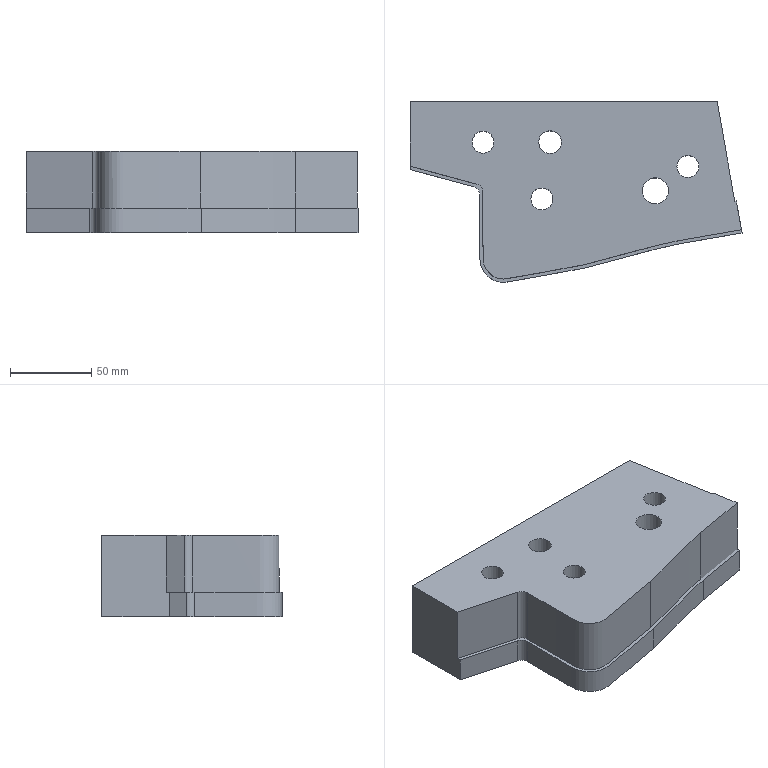Part | NX | features solid 2 | 1 solid | 32 faces | box 204.747 x 111.347 x 50 mm | volume 704636 mm3 | plane 16 | cylinder 10 | spline 6 | commonest cylinder face diameters 13.5 x3 19.5 x3 10 x2 14 x1 16 x1
STEP:
#1=CARTESIAN_POINT('',(-1121.897,435.,3.));
#2=VERTEX_POINT('',#1);
#3=CARTESIAN_POINT('',(-1121.897,435.,43.));
#4=VERTEX_POINT('',#3);
#5=CARTESIAN_POINT('',(-1121.897,435.,-60.));
#6=DIRECTION('',(0.,0.,-1.));
#7=VECTOR('',#6,1000.);
#8=LINE('',#5,#7);
#9=EDGE_CURVE('',#2,#4,#8,.F.);
#10=ORIENTED_EDGE('',*,*,#9,.F.);
#11=CARTESIAN_POINT('',(-1243.358,435.,3.));
#12=VERTEX_POINT('',#11);
#13=CARTESIAN_POINT('',(-1263.358,435.,3.));
#14=DIRECTION('',(-1.,0.,0.));
#15=VECTOR('',#14,1000.);
#16=LINE('',#13,#15);
#17=EDGE_CURVE('',#12,#2,#16,.F.);
#18=ORIENTED_EDGE('',*,*,#17,.F.);
#19=CARTESIAN_POINT('',(-1243.358,435.,-7.));
#20=VERTEX_POINT('',#19);
#21=CARTESIAN_POINT('',(-1243.358,435.,3.));
#22=DIRECTION('',(0.,0.,1.));
#23=VECTOR('',#22,1000.);
#24=LINE('',#21,#23);
#25=EDGE_CURVE('',#12,#20,#24,.F.);
#26=ORIENTED_EDGE('',*,*,#25,.T.);
#27=CARTESIAN_POINT('',(-1311.358,435.,-7.));
#28=VERTEX_POINT('',#27);
#29=CARTESIAN_POINT('',(-1263.358,435.,-7.));
#30=DIRECTION('',(-1.,0.,0.));
#31=VECTOR('',#30,1000.);
#32=LINE('',#29,#31);
#33=EDGE_CURVE('',#28,#20,#32,.F.);
#34=ORIENTED_EDGE('',*,*,#33,.F.);
#35=CARTESIAN_POINT('',(-1311.358,435.,43.));
#36=VERTEX_POINT('',#35);
#37=CARTESIAN_POINT('',(-1311.358,435.,-60.));
#38=DIRECTION('',(0.,0.,-1.));
#39=VECTOR('',#38,1000.);
#40=LINE('',#37,#39);
#41=EDGE_CURVE('',#36,#28,#40,.T.);
#42=ORIENTED_EDGE('',*,*,#41,.F.);
#43=CARTESIAN_POINT('',(-1263.358,435.,43.));
#44=DIRECTION('',(-1.,0.,0.));
#45=VECTOR('',#44,1000.);
#46=LINE('',#43,#45);
#47=EDGE_CURVE('',#36,#4,#46,.F.);
#48=ORIENTED_EDGE('',*,*,#47,.T.);
#49=EDGE_LOOP('',(#10,#18,#26,#34,#42,#48));
#50=FACE_BOUND('',#49,.T.);
#51=CARTESIAN_POINT('',(-1263.358,435.,-60.));
#52=DIRECTION('',(0.,1.,0.));
#53=DIRECTION('',(-1.,0.,0.));
#54=AXIS2_PLACEMENT_3D('',#51,#52,#53);
#55=PLANE('',#54);
#56=ADVANCED_FACE('',(#50),#55,.T.);
#57=CARTESIAN_POINT('',(-1266.355,379.299,8.));
#58=VERTEX_POINT('',#57);
#59=CARTESIAN_POINT('',(-1203.794,334.49,8.));
#60=VERTEX_POINT('',#59);
#61=CARTESIAN_POINT('',(-1266.355,379.299,8.));
#62=CARTESIAN_POINT('',(-1266.355,376.959,8.));
#63=CARTESIAN_POINT('',(-1266.356,372.279,8.));
#64=CARTESIAN_POINT('',(-1266.359,365.259,8.));
#65=CARTESIAN_POINT('',(-1266.363,358.239,8.));
#66=CARTESIAN_POINT('',(-1266.367,352.389,8.));
#67=CARTESIAN_POINT('',(-1266.372,347.71,8.));
#68=CARTESIAN_POINT('',(-1266.376,344.199,8.));
#69=CARTESIAN_POINT('',(-1266.38,340.694,8.));
#70=CARTESIAN_POINT('',(-1266.398,337.165,8.));
#71=CARTESIAN_POINT('',(-1265.599,333.731,8.));
#72=CARTESIAN_POINT('',(-1263.894,330.627,8.));
#73=CARTESIAN_POINT('',(-1261.439,328.077,8.));
#74=CARTESIAN_POINT('',(-1258.382,326.304,8.));
#75=CARTESIAN_POINT('',(-1254.93,325.476,8.));
#76=CARTESIAN_POINT('',(-1251.442,325.852,8.));
#77=CARTESIAN_POINT('',(-1248.056,326.515,8.));
#78=CARTESIAN_POINT('',(-1243.504,327.281,8.));
#79=CARTESIAN_POINT('',(-1237.826,328.278,8.));
#80=CARTESIAN_POINT('',(-1231.005,329.449,8.));
#81=CARTESIAN_POINT('',(-1224.186,330.621,8.));
#82=CARTESIAN_POINT('',(-1215.094,332.188,8.));
#83=CARTESIAN_POINT('',(-1208.297,333.483,8.));
#84=CARTESIAN_POINT('',(-1203.794,334.49,8.));
#85=B_SPLINE_CURVE_WITH_KNOTS('',3,(#61,#62,#63,#64,#65,#66,#67,#68,#69,#70,#71,#72,#73,#74,#75,#76,#77,#78,#79,#80,#81,#82,#83,#84),.UNSPECIFIED.,.F.,.F.,(4,1,1,1,1,1,1,1,1,1,1,1,1,1,1,1,1,1,1,1,1,4),(0.0507,0.05772,0.06474,0.07176,0.07878,0.08229,0.0858,0.08931,0.09282,0.09633,0.09984,0.1033,0.1069,0.1104,0.1139,0.1174,0.1209,0.1279,0.1349,0.142,0.149,0.163),.UNSPECIFIED.);
#86=EDGE_CURVE('',#58,#60,#85,.T.);
#87=ORIENTED_EDGE('',*,*,#86,.F.);
#88=CARTESIAN_POINT('',(-1270.061,384.129,8.));
#89=VERTEX_POINT('',#88);
#90=CARTESIAN_POINT('',(-1271.355,379.3,8.));
#91=DIRECTION('',(0.,0.,1.));
#92=DIRECTION('',(1.,0.,0.));
#93=AXIS2_PLACEMENT_3D('',#90,#91,#92);
#94=CIRCLE('',#93,5.);
#95=EDGE_CURVE('',#58,#89,#94,.T.);
#96=ORIENTED_EDGE('',*,*,#95,.T.);
#97=CARTESIAN_POINT('',(-1311.358,395.195,8.));
#98=VERTEX_POINT('',#97);
#99=CARTESIAN_POINT('',(-1243.118,376.91,8.));
#100=DIRECTION('',(0.9659,-0.2588,0.));
#101=VECTOR('',#100,1000.);
#102=LINE('',#99,#101);
#103=EDGE_CURVE('',#89,#98,#102,.F.);
#104=ORIENTED_EDGE('',*,*,#103,.T.);
#105=CARTESIAN_POINT('',(-1311.358,393.124,8.));
#106=VERTEX_POINT('',#105);
#107=CARTESIAN_POINT('',(-1311.358,338.697,8.));
#108=DIRECTION('',(0.,1.,0.));
#109=VECTOR('',#108,1000.);
#110=LINE('',#107,#109);
#111=EDGE_CURVE('',#98,#106,#110,.F.);
#112=ORIENTED_EDGE('',*,*,#111,.T.);
#113=CARTESIAN_POINT('',(-1272.064,382.595,8.));
#114=VERTEX_POINT('',#113);
#115=CARTESIAN_POINT('',(-1318.358,395.,8.));
#116=DIRECTION('',(0.9659,-0.2588,0.));
#117=VECTOR('',#116,1000.);
#118=LINE('',#115,#117);
#119=EDGE_CURVE('',#114,#106,#118,.F.);
#120=ORIENTED_EDGE('',*,*,#119,.F.);
#121=CARTESIAN_POINT('',(-1268.358,377.765,8.));
#122=VERTEX_POINT('',#121);
#123=CARTESIAN_POINT('',(-1273.358,377.766,8.));
#124=DIRECTION('',(0.,0.,1.));
#125=DIRECTION('',(1.,0.,0.));
#126=AXIS2_PLACEMENT_3D('',#123,#124,#125);
#127=CIRCLE('',#126,5.);
#128=EDGE_CURVE('',#114,#122,#127,.F.);
#129=ORIENTED_EDGE('',*,*,#128,.T.);
#130=CARTESIAN_POINT('',(-1203.358,332.538,8.));
#131=VERTEX_POINT('',#130);
#132=CARTESIAN_POINT('',(-1268.358,377.765,8.));
#133=CARTESIAN_POINT('',(-1268.358,375.398,8.));
#134=CARTESIAN_POINT('',(-1268.359,370.662,8.));
#135=CARTESIAN_POINT('',(-1268.362,363.558,8.));
#136=CARTESIAN_POINT('',(-1268.362,356.456,8.));
#137=CARTESIAN_POINT('',(-1268.38,349.349,8.));
#138=CARTESIAN_POINT('',(-1268.342,342.262,8.));
#139=CARTESIAN_POINT('',(-1268.525,335.095,8.));
#140=CARTESIAN_POINT('',(-1265.854,329.641,8.));
#141=CARTESIAN_POINT('',(-1262.445,326.353,8.));
#142=CARTESIAN_POINT('',(-1259.354,324.562,8.));
#143=CARTESIAN_POINT('',(-1255.924,323.61,8.));
#144=CARTESIAN_POINT('',(-1252.369,323.625,8.));
#145=CARTESIAN_POINT('',(-1248.874,324.351,8.));
#146=CARTESIAN_POINT('',(-1245.366,324.93,8.));
#147=CARTESIAN_POINT('',(-1241.862,325.548,8.));
#148=CARTESIAN_POINT('',(-1237.188,326.357,8.));
#149=CARTESIAN_POINT('',(-1229.008,327.775,8.));
#150=CARTESIAN_POINT('',(-1217.313,329.745,8.));
#151=CARTESIAN_POINT('',(-1207.99,331.502,8.));
#152=CARTESIAN_POINT('',(-1203.358,332.538,8.));
#153=B_SPLINE_CURVE_WITH_KNOTS('',3,(#132,#133,#134,#135,#136,#137,#138,#139,#140,#141,#142,#143,#144,#145,#146,#147,#148,#149,#150,#151,#152),.UNSPECIFIED.,.F.,.F.,(4,1,1,1,1,1,1,1,1,1,1,1,1,1,1,1,1,1,4),(0.05223,0.05934,0.06644,0.07354,0.08065,0.08775,0.09485,0.102,0.1055,0.1091,0.1126,0.1162,0.1197,0.1233,0.1268,0.1304,0.1375,0.1517,0.1659),.UNSPECIFIED.);
#154=EDGE_CURVE('',#122,#131,#153,.T.);
#155=ORIENTED_EDGE('',*,*,#154,.T.);
#156=CARTESIAN_POINT('',(-1145.033,347.385,8.));
#157=VERTEX_POINT('',#156);
#158=CARTESIAN_POINT('',(-1145.033,347.385,8.));
#159=CARTESIAN_POINT('',(-1154.893,345.514,8.));
#160=CARTESIAN_POINT('',(-1174.32,340.449,8.));
#161=CARTESIAN_POINT('',(-1193.559,334.73,8.));
#162=CARTESIAN_POINT('',(-1203.358,332.538,8.));
#163=B_SPLINE_CURVE_WITH_KNOTS('',3,(#158,#159,#160,#161,#162),.UNSPECIFIED.,.F.,.F.,(4,1,4),(0.,0.03009,0.06019),.UNSPECIFIED.);
#164=EDGE_CURVE('',#157,#131,#163,.T.);
#165=ORIENTED_EDGE('',*,*,#164,.F.);
#166=CARTESIAN_POINT('',(-1106.611,354.067,8.));
#167=VERTEX_POINT('',#166);
#168=CARTESIAN_POINT('',(-1145.033,347.385,8.));
#169=CARTESIAN_POINT('',(-1132.226,349.613,8.));
#170=CARTESIAN_POINT('',(-1119.418,351.84,8.));
#171=CARTESIAN_POINT('',(-1106.611,354.067,8.));
#172=B_SPLINE_CURVE_WITH_KNOTS('',3,(#168,#169,#170,#171),.UNSPECIFIED.,.F.,.F.,(4,4),(1.708,1.747),.UNSPECIFIED.);
#173=EDGE_CURVE('',#157,#167,#172,.T.);
#174=ORIENTED_EDGE('',*,*,#173,.T.);
#175=CARTESIAN_POINT('',(-1106.959,356.038,8.));
#176=VERTEX_POINT('',#175);
#177=CARTESIAN_POINT('',(-1108.407,364.255,8.));
#178=DIRECTION('',(0.1736,-0.9848,0.));
#179=VECTOR('',#178,1000.);
#180=LINE('',#177,#179);
#181=EDGE_CURVE('',#176,#167,#180,.T.);
#182=ORIENTED_EDGE('',*,*,#181,.F.);
#183=CARTESIAN_POINT('',(-1145.406,349.351,8.));
#184=VERTEX_POINT('',#183);
#185=CARTESIAN_POINT('',(-1145.406,349.351,8.));
#186=CARTESIAN_POINT('',(-1132.59,351.58,8.));
#187=CARTESIAN_POINT('',(-1119.774,353.809,8.));
#188=CARTESIAN_POINT('',(-1106.959,356.038,8.));
#189=B_SPLINE_CURVE_WITH_KNOTS('',3,(#185,#186,#187,#188),.UNSPECIFIED.,.F.,.F.,(4,4),(1.656,1.695),.UNSPECIFIED.);
#190=EDGE_CURVE('',#184,#176,#189,.T.);
#191=ORIENTED_EDGE('',*,*,#190,.F.);
#192=CARTESIAN_POINT('',(-1145.406,349.35,8.));
#193=VERTEX_POINT('',#192);
#194=CARTESIAN_POINT('',(-1145.033,347.385,8.));
#195=DIRECTION('',(-0.1865,0.9825,0.));
#196=VECTOR('',#195,1000.);
#197=LINE('',#194,#196);
#198=EDGE_CURVE('',#193,#184,#197,.T.);
#199=ORIENTED_EDGE('',*,*,#198,.F.);
#200=CARTESIAN_POINT('',(-1145.406,349.35,8.));
#201=CARTESIAN_POINT('',(-1155.28,347.476,8.));
#202=CARTESIAN_POINT('',(-1174.721,342.418,8.));
#203=CARTESIAN_POINT('',(-1193.989,336.683,8.));
#204=CARTESIAN_POINT('',(-1203.794,334.49,8.));
#205=B_SPLINE_CURVE_WITH_KNOTS('',3,(#200,#201,#202,#203,#204),.UNSPECIFIED.,.F.,.F.,(4,1,4),(0.2409,0.271,0.3012),.UNSPECIFIED.);
#206=EDGE_CURVE('',#193,#60,#205,.T.);
#207=ORIENTED_EDGE('',*,*,#206,.T.);
#208=EDGE_LOOP('',(#87,#96,#104,#112,#120,#129,#155,#165,#174,#182,#191,#199,#207));
#209=FACE_BOUND('',#208,.T.);
#210=CARTESIAN_POINT('',(-1253.358,338.697,8.));
#211=DIRECTION('',(0.,0.,1.));
#212=DIRECTION('',(1.,0.,0.));
#213=AXIS2_PLACEMENT_3D('',#210,#211,#212);
#214=PLANE('',#213);
#215=ADVANCED_FACE('',(#209),#214,.T.);
#216=ORIENTED_EDGE('',*,*,#154,.F.);
#217=CARTESIAN_POINT('',(-1268.358,377.765,-7.));
#218=VERTEX_POINT('',#217);
#219=CARTESIAN_POINT('',(-1268.358,377.765,8.));
#220=DIRECTION('',(0.,0.,1.));
#221=VECTOR('',#220,1000.);
#222=LINE('',#219,#221);
#223=EDGE_CURVE('',#122,#218,#222,.F.);
#224=ORIENTED_EDGE('',*,*,#223,.T.);
#225=CARTESIAN_POINT('',(-1203.358,332.538,-7.));
#226=VERTEX_POINT('',#225);
#227=CARTESIAN_POINT('',(-1268.358,377.765,-7.));
#228=CARTESIAN_POINT('',(-1268.358,375.398,-7.));
#229=CARTESIAN_POINT('',(-1268.359,370.662,-7.));
#230=CARTESIAN_POINT('',(-1268.362,363.558,-7.));
#231=CARTESIAN_POINT('',(-1268.362,356.456,-7.));
#232=CARTESIAN_POINT('',(-1268.38,349.349,-7.));
#233=CARTESIAN_POINT('',(-1268.342,342.262,-7.));
#234=CARTESIAN_POINT('',(-1268.525,335.095,-7.));
#235=CARTESIAN_POINT('',(-1265.854,329.641,-7.));
#236=CARTESIAN_POINT('',(-1262.445,326.353,-7.));
#237=CARTESIAN_POINT('',(-1259.354,324.562,-7.));
#238=CARTESIAN_POINT('',(-1255.924,323.61,-7.));
#239=CARTESIAN_POINT('',(-1252.369,323.625,-7.));
#240=CARTESIAN_POINT('',(-1248.874,324.351,-7.));
#241=CARTESIAN_POINT('',(-1245.366,324.93,-7.));
#242=CARTESIAN_POINT('',(-1241.862,325.548,-7.));
#243=CARTESIAN_POINT('',(-1237.188,326.357,-7.));
#244=CARTESIAN_POINT('',(-1229.008,327.775,-7.));
#245=CARTESIAN_POINT('',(-1217.313,329.745,-7.));
#246=CARTESIAN_POINT('',(-1207.99,331.502,-7.));
#247=CARTESIAN_POINT('',(-1203.358,332.538,-7.));
#248=B_SPLINE_CURVE_WITH_KNOTS('',3,(#227,#228,#229,#230,#231,#232,#233,#234,#235,#236,#237,#238,#239,#240,#241,#242,#243,#244,#245,#246,#247),.UNSPECIFIED.,.F.,.F.,(4,1,1,1,1,1,1,1,1,1,1,1,1,1,1,1,1,1,4),(0.05223,0.05934,0.06644,0.07354,0.08065,0.08775,0.09485,0.102,0.1055,0.1091,0.1126,0.1162,0.1197,0.1233,0.1268,0.1304,0.1375,0.1517,0.1659),.UNSPECIFIED.);
#249=EDGE_CURVE('',#218,#226,#248,.T.);
#250=ORIENTED_EDGE('',*,*,#249,.T.);
#251=CARTESIAN_POINT('',(-1203.358,332.538,-100.));
#252=DIRECTION('',(0.,0.,1.));
#253=VECTOR('',#252,1000.);
#254=LINE('',#251,#253);
#255=EDGE_CURVE('',#131,#226,#254,.F.);
#256=ORIENTED_EDGE('',*,*,#255,.F.);
#257=EDGE_LOOP('',(#216,#224,#250,#256));
#258=FACE_BOUND('',#257,.T.);
#259=CARTESIAN_POINT('',(-1268.358,377.765,-7.));
#260=CARTESIAN_POINT('',(-1268.358,377.765,8.));
#261=CARTESIAN_POINT('',(-1268.358,375.398,-7.));
#262=CARTESIAN_POINT('',(-1268.358,375.398,8.));
#263=CARTESIAN_POINT('',(-1268.359,370.665,-7.));
#264=CARTESIAN_POINT('',(-1268.359,370.665,8.));
#265=CARTESIAN_POINT('',(-1268.362,363.564,-7.));
#266=CARTESIAN_POINT('',(-1268.362,363.564,8.));
#267=CARTESIAN_POINT('',(-1268.362,356.465,-7.));
#268=CARTESIAN_POINT('',(-1268.362,356.465,8.));
#269=CARTESIAN_POINT('',(-1268.38,349.357,-7.));
#270=CARTESIAN_POINT('',(-1268.38,349.357,8.));
#271=CARTESIAN_POINT('',(-1268.341,342.281,-7.));
#272=CARTESIAN_POINT('',(-1268.341,342.281,8.));
#273=CARTESIAN_POINT('',(-1268.527,335.088,-7.));
#274=CARTESIAN_POINT('',(-1268.527,335.088,8.));
#275=CARTESIAN_POINT('',(-1265.301,328.509,-7.));
#276=CARTESIAN_POINT('',(-1265.301,328.509,8.));
#277=CARTESIAN_POINT('',(-1260.437,324.845,-7.));
#278=CARTESIAN_POINT('',(-1260.437,324.845,8.));
#279=CARTESIAN_POINT('',(-1255.829,323.594,-7.));
#280=CARTESIAN_POINT('',(-1255.829,323.594,8.));
#281=CARTESIAN_POINT('',(-1252.254,323.645,-7.));
#282=CARTESIAN_POINT('',(-1252.254,323.645,8.));
#283=CARTESIAN_POINT('',(-1248.771,324.369,-7.));
#284=CARTESIAN_POINT('',(-1248.771,324.369,8.));
#285=CARTESIAN_POINT('',(-1245.269,324.947,-7.));
#286=CARTESIAN_POINT('',(-1245.269,324.947,8.));
#287=CARTESIAN_POINT('',(-1241.772,325.563,-7.));
#288=CARTESIAN_POINT('',(-1241.772,325.563,8.));
#289=CARTESIAN_POINT('',(-1237.108,326.37,-7.));
#290=CARTESIAN_POINT('',(-1237.108,326.37,8.));
#291=CARTESIAN_POINT('',(-1228.945,327.786,-7.));
#292=CARTESIAN_POINT('',(-1228.945,327.786,8.));
#293=CARTESIAN_POINT('',(-1217.272,329.752,-7.));
#294=CARTESIAN_POINT('',(-1217.272,329.752,8.));
#295=CARTESIAN_POINT('',(-1207.973,331.506,-7.));
#296=CARTESIAN_POINT('',(-1207.973,331.506,8.));
#297=CARTESIAN_POINT('',(-1203.358,332.538,-7.));
#298=CARTESIAN_POINT('',(-1203.358,332.538,8.));
#299=B_SPLINE_SURFACE_WITH_KNOTS('',3,1,((#259,#260),(#261,#262),(#263,#264),(#265,#266),(#267,#268),(#269,#270),(#271,#272),(#273,#274),(#275,#276),(#277,#278),(#279,#280),(#281,#282),(#283,#284),(#285,#286),(#287,#288),(#289,#290),(#291,#292),(#293,#294),(#295,#296),(#297,#298)),.SURF_OF_LINEAR_EXTRUSION.,.F.,.F.,.F.,(4,1,1,1,1,1,1,1,1,1,1,1,1,1,1,1,1,4),(2,2),(0.1341,0.1494,0.1647,0.18,0.1953,0.2106,0.2259,0.2413,0.2566,0.2642,0.2719,0.2795,0.2872,0.2948,0.3025,0.3178,0.3484,0.379),(0.,1.),.UNSPECIFIED.);
#300=ADVANCED_FACE('',(#258),#299,.T.);
#301=CARTESIAN_POINT('',(-1266.355,379.299,43.));
#302=VERTEX_POINT('',#301);
#303=CARTESIAN_POINT('',(-1203.794,334.49,43.));
#304=VERTEX_POINT('',#303);
#305=CARTESIAN_POINT('',(-1266.355,379.299,43.));
#306=CARTESIAN_POINT('',(-1266.355,376.955,43.));
#307=CARTESIAN_POINT('',(-1266.356,372.268,43.));
#308=CARTESIAN_POINT('',(-1266.359,365.238,43.));
#309=CARTESIAN_POINT('',(-1266.363,358.207,43.));
#310=CARTESIAN_POINT('',(-1266.367,352.348,43.));
#311=CARTESIAN_POINT('',(-1266.372,347.662,43.));
#312=CARTESIAN_POINT('',(-1266.376,344.145,43.));
#313=CARTESIAN_POINT('',(-1266.382,340.636,43.));
#314=CARTESIAN_POINT('',(-1266.393,337.097,43.));
#315=CARTESIAN_POINT('',(-1265.577,333.676,43.));
#316=CARTESIAN_POINT('',(-1263.86,330.581,43.));
#317=CARTESIAN_POINT('',(-1261.394,328.043,43.));
#318=CARTESIAN_POINT('',(-1258.33,326.283,43.));
#319=CARTESIAN_POINT('',(-1254.87,325.472,43.));
#320=CARTESIAN_POINT('',(-1251.394,325.864,43.));
#321=CARTESIAN_POINT('',(-1248.01,326.522,43.));
#322=CARTESIAN_POINT('',(-1243.462,327.289,43.));
#323=CARTESIAN_POINT('',(-1237.79,328.284,43.));
#324=CARTESIAN_POINT('',(-1230.977,329.454,43.));
#325=CARTESIAN_POINT('',(-1224.164,330.625,43.));
#326=CARTESIAN_POINT('',(-1215.081,332.191,43.));
#327=CARTESIAN_POINT('',(-1208.292,333.484,43.));
#328=CARTESIAN_POINT('',(-1203.794,334.49,43.));
#329=B_SPLINE_CURVE_WITH_KNOTS('',3,(#305,#306,#307,#308,#309,#310,#311,#312,#313,#314,#315,#316,#317,#318,#319,#320,#321,#322,#323,#324,#325,#326,#327,#328),.UNSPECIFIED.,.F.,.F.,(4,1,1,1,1,1,1,1,1,1,1,1,1,1,1,1,1,1,1,1,1,4),(0.7322,0.7393,0.7463,0.7533,0.7604,0.7639,0.7674,0.7709,0.7744,0.7779,0.7814,0.785,0.7885,0.792,0.7955,0.799,0.8025,0.8096,0.8166,0.8236,0.8307,0.8447),.UNSPECIFIED.);
#330=EDGE_CURVE('',#302,#304,#329,.T.);
#331=ORIENTED_EDGE('',*,*,#330,.F.);
#332=CARTESIAN_POINT('',(-1266.355,379.299,43.));
#333=DIRECTION('',(0.,0.,-1.));
#334=VECTOR('',#333,1000.);
#335=LINE('',#332,#334);
#336=EDGE_CURVE('',#302,#58,#335,.T.);
#337=ORIENTED_EDGE('',*,*,#336,.T.);
#338=ORIENTED_EDGE('',*,*,#86,.T.);
#339=CARTESIAN_POINT('',(-1203.794,334.49,24.5));
#340=DIRECTION('',(0.,0.,-1.));
#341=VECTOR('',#340,1000.);
#342=LINE('',#339,#341);
#343=EDGE_CURVE('',#60,#304,#342,.F.);
#344=ORIENTED_EDGE('',*,*,#343,.T.);
#345=EDGE_LOOP('',(#331,#337,#338,#344));
#346=FACE_BOUND('',#345,.T.);
#347=CARTESIAN_POINT('',(-1266.355,379.299,43.));
#348=CARTESIAN_POINT('',(-1266.355,379.299,8.));
#349=CARTESIAN_POINT('',(-1266.356,374.499,43.));
#350=CARTESIAN_POINT('',(-1266.356,374.499,8.));
#351=CARTESIAN_POINT('',(-1266.358,367.298,43.));
#352=CARTESIAN_POINT('',(-1266.358,367.298,8.));
#353=CARTESIAN_POINT('',(-1266.362,357.703,43.));
#354=CARTESIAN_POINT('',(-1266.362,357.703,8.));
#355=CARTESIAN_POINT('',(-1266.374,350.489,43.));
#356=CARTESIAN_POINT('',(-1266.374,350.489,8.));
#357=CARTESIAN_POINT('',(-1266.36,344.535,43.));
#358=CARTESIAN_POINT('',(-1266.36,344.535,8.));
#359=CARTESIAN_POINT('',(-1266.409,339.641,43.));
#360=CARTESIAN_POINT('',(-1266.409,339.641,8.));
#361=CARTESIAN_POINT('',(-1266.285,336.407,43.));
#362=CARTESIAN_POINT('',(-1266.285,336.407,8.));
#363=CARTESIAN_POINT('',(-1265.43,333.419,43.));
#364=CARTESIAN_POINT('',(-1265.43,333.419,8.));
#365=CARTESIAN_POINT('',(-1263.391,329.775,43.));
#366=CARTESIAN_POINT('',(-1263.391,329.775,8.));
#367=CARTESIAN_POINT('',(-1260.122,327.015,43.));
#368=CARTESIAN_POINT('',(-1260.122,327.015,8.));
#369=CARTESIAN_POINT('',(-1256.764,325.885,43.));
#370=CARTESIAN_POINT('',(-1256.764,325.885,8.));
#371=CARTESIAN_POINT('',(-1254.702,325.628,43.));
#372=CARTESIAN_POINT('',(-1254.702,325.628,8.));
#373=CARTESIAN_POINT('',(-1253.207,325.641,43.));
#374=CARTESIAN_POINT('',(-1253.207,325.641,8.));
#375=CARTESIAN_POINT('',(-1251.619,325.86,43.));
#376=CARTESIAN_POINT('',(-1251.619,325.86,8.));
#377=CARTESIAN_POINT('',(-1249.242,326.301,43.));
#378=CARTESIAN_POINT('',(-1249.242,326.301,8.));
#379=CARTESIAN_POINT('',(-1246.274,326.806,43.));
#380=CARTESIAN_POINT('',(-1246.274,326.806,8.));
#381=CARTESIAN_POINT('',(-1242.725,327.426,43.));
#382=CARTESIAN_POINT('',(-1242.725,327.426,8.));
#383=CARTESIAN_POINT('',(-1237.984,328.246,43.));
#384=CARTESIAN_POINT('',(-1237.984,328.246,8.));
#385=CARTESIAN_POINT('',(-1229.696,329.68,43.));
#386=CARTESIAN_POINT('',(-1229.696,329.68,8.));
#387=CARTESIAN_POINT('',(-1217.814,331.684,43.));
#388=CARTESIAN_POINT('',(-1217.814,331.684,8.));
#389=CARTESIAN_POINT('',(-1208.489,333.44,43.));
#390=CARTESIAN_POINT('',(-1208.489,333.44,8.));
#391=CARTESIAN_POINT('',(-1203.794,334.49,43.));
#392=CARTESIAN_POINT('',(-1203.794,334.49,8.));
#393=B_SPLINE_SURFACE_WITH_KNOTS('',3,1,((#347,#348),(#349,#350),(#351,#352),(#353,#354),(#355,#356),(#357,#358),(#359,#360),(#361,#362),(#363,#364),(#365,#366),(#367,#368),(#369,#370),(#371,#372),(#373,#374),(#375,#376),(#377,#378),(#379,#380),(#381,#382),(#383,#384),(#385,#386),(#387,#388),(#389,#390),(#391,#392)),.SURF_OF_LINEAR_EXTRUSION.,.F.,.F.,.F.,(4,1,1,1,1,1,1,1,1,1,1,1,1,1,1,1,1,1,1,1,4),(2,2),(0.3056,0.3924,0.4358,0.4792,0.5226,0.5443,0.566,0.5877,0.6094,0.6528,0.6745,0.6854,0.6962,0.7071,0.7179,0.7396,0.7613,0.783,0.8264,0.9132,1.),(0.,1.),.UNSPECIFIED.);
#394=ADVANCED_FACE('',(#346),#393,.F.);
#395=CARTESIAN_POINT('',(-1145.033,347.385,-7.));
#396=VERTEX_POINT('',#395);
#397=CARTESIAN_POINT('',(-1145.033,347.385,-7.));
#398=DIRECTION('',(0.,0.,1.));
#399=VECTOR('',#398,1000.);
#400=LINE('',#397,#399);
#401=EDGE_CURVE('',#396,#157,#400,.T.);
#402=ORIENTED_EDGE('',*,*,#401,.F.);
#403=CARTESIAN_POINT('',(-1106.611,354.067,-7.));
#404=VERTEX_POINT('',#403);
#405=CARTESIAN_POINT('',(-1263.358,326.807,-7.));
#406=CARTESIAN_POINT('',(-1232.991,332.088,-7.));
#407=CARTESIAN_POINT('',(-1171.809,342.729,-7.));
#408=CARTESIAN_POINT('',(-1095.22,356.049,-7.));
#409=CARTESIAN_POINT('',(-1033.589,366.767,-7.));
#410=CARTESIAN_POINT('',(-987.365,374.804,-7.));
#411=CARTESIAN_POINT('',(-948.847,381.509,-7.));
#412=CARTESIAN_POINT('',(-923.808,385.853,-7.));
#413=CARTESIAN_POINT('',(-914.109,387.486,-7.));
#414=CARTESIAN_POINT('',(-912.091,387.827,-7.));
#415=CARTESIAN_POINT('',(-911.971,387.848,-7.));
#416=CARTESIAN_POINT('',(-911.79,387.876,-7.));
#417=CARTESIAN_POINT('',(-911.394,387.917,-7.));
#418=CARTESIAN_POINT('',(-910.546,388.022,-7.));
#419=CARTESIAN_POINT('',(-908.847,388.221,-7.));
#420=CARTESIAN_POINT('',(-906.42,388.511,-7.));
#421=CARTESIAN_POINT('',(-903.994,388.799,-7.));
#422=CARTESIAN_POINT('',(-902.295,389.001,-7.));
#423=CARTESIAN_POINT('',(-901.446,389.101,-7.));
#424=CARTESIAN_POINT('',(-901.052,389.148,-7.));
#425=CARTESIAN_POINT('',(-900.87,389.17,-7.));
#426=CARTESIAN_POINT('',(-900.748,389.184,-7.));
#427=CARTESIAN_POINT('',(-899.68,389.239,-7.));
#428=CARTESIAN_POINT('',(-897.973,389.35,-7.));
#429=CARTESIAN_POINT('',(-896.023,389.486,-7.));
#430=CARTESIAN_POINT('',(-894.456,389.561,-7.));
#431=CARTESIAN_POINT('',(-892.989,389.903,-7.));
#432=CARTESIAN_POINT('',(-891.495,390.907,-7.));
#433=CARTESIAN_POINT('',(-890.458,392.378,-7.));
#434=CARTESIAN_POINT('',(-890.077,393.863,-7.));
#435=CARTESIAN_POINT('',(-889.825,397.101,-7.));
#436=CARTESIAN_POINT('',(-889.362,402.393,-7.));
#437=CARTESIAN_POINT('',(-888.928,407.354,-7.));
#438=CARTESIAN_POINT('',(-888.696,410.,-7.));
#439=B_SPLINE_CURVE_WITH_KNOTS('',3,(#405,#406,#407,#408,#409,#410,#411,#412,#413,#414,#415,#416,#417,#418,#419,#420,#421,#422,#423,#424,#425,#426,#427,#428,#429,#430,#431,#432,#433,#434,#435,#436,#437,#438),.UNSPECIFIED.,.F.,.F.,(4,1,1,1,1,1,1,1,1,1,1,1,1,1,1,1,1,1,1,1,1,1,1,1,1,1,1,1,1,1,1,4),(0.,0.2329,0.4693,0.5875,0.7056,0.8238,0.8829,0.8977,0.8981,0.8984,0.8986,0.8995,0.9014,0.9051,0.9124,0.9198,0.9235,0.9254,0.9263,0.9265,0.9268,0.9272,0.9346,0.9397,0.942,0.9465,0.9509,0.9554,0.9599,0.9624,0.9799,1.),.UNSPECIFIED.);
#440=EDGE_CURVE('',#396,#404,#439,.T.);
#441=ORIENTED_EDGE('',*,*,#440,.T.);
#442=CARTESIAN_POINT('',(-1106.611,354.067,0.5));
#443=DIRECTION('',(0.,0.,-1.));
#444=VECTOR('',#443,1000.);
#445=LINE('',#442,#444);
#446=EDGE_CURVE('',#404,#167,#445,.F.);
#447=ORIENTED_EDGE('',*,*,#446,.T.);
#448=ORIENTED_EDGE('',*,*,#173,.F.);
#449=EDGE_LOOP('',(#402,#441,#447,#448));
#450=FACE_BOUND('',#449,.T.);
#451=CARTESIAN_POINT('',(-1145.033,347.385,8.));
#452=CARTESIAN_POINT('',(-1145.033,347.385,-7.));
#453=CARTESIAN_POINT('',(-1132.226,349.613,8.));
#454=CARTESIAN_POINT('',(-1132.226,349.613,-7.));
#455=CARTESIAN_POINT('',(-1119.418,351.84,8.));
#456=CARTESIAN_POINT('',(-1119.418,351.84,-7.));
#457=CARTESIAN_POINT('',(-1106.611,354.067,8.));
#458=CARTESIAN_POINT('',(-1106.611,354.067,-7.));
#459=B_SPLINE_SURFACE_WITH_KNOTS('',3,1,((#451,#452),(#453,#454),(#455,#456),(#457,#458)),.SURF_OF_LINEAR_EXTRUSION.,.F.,.F.,.F.,(4,4),(2,2),(0.3025,0.4008),(0.,1.),.PIECEWISE_BEZIER_KNOTS.);
#460=ADVANCED_FACE('',(#450),#459,.F.);
#461=CARTESIAN_POINT('',(-1256.608,410.,-7.));
#462=VERTEX_POINT('',#461);
#463=CARTESIAN_POINT('',(-1266.358,410.,-7.));
#464=DIRECTION('',(0.,0.,1.));
#465=DIRECTION('',(1.,0.,0.));
#466=AXIS2_PLACEMENT_3D('',#463,#464,#465);
#467=CIRCLE('',#466,9.75);
#468=EDGE_CURVE('',#462,#462,#467,.T.);
#469=ORIENTED_EDGE('',*,*,#468,.T.);
#470=EDGE_LOOP('',(#469));
#471=FACE_BOUND('',#470,.T.);
#472=ORIENTED_EDGE('',*,*,#33,.T.);
#473=CARTESIAN_POINT('',(-1243.358,350.586,-7.));
#474=VERTEX_POINT('',#473);
#475=CARTESIAN_POINT('',(-1243.358,441.912,-7.));
#476=CARTESIAN_POINT('',(-1243.358,437.941,-7.));
#477=CARTESIAN_POINT('',(-1243.358,433.971,-7.));
#478=CARTESIAN_POINT('',(-1243.358,430.,-7.));
#479=CARTESIAN_POINT('',(-1243.358,403.529,-7.));
#480=CARTESIAN_POINT('',(-1243.358,377.057,-7.));
#481=CARTESIAN_POINT('',(-1243.358,350.586,-7.));
#482=CARTESIAN_POINT('',(-1243.358,346.615,-7.));
#483=CARTESIAN_POINT('',(-1243.358,342.644,-7.));
#484=CARTESIAN_POINT('',(-1243.358,338.674,-7.));
#485=B_SPLINE_CURVE_WITH_KNOTS('',3,(#475,#476,#477,#478,#479,#480,#481,#482,#483,#484),.UNSPECIFIED.,.F.,.F.,(4,3,3,4),(-0.05549,0.,0.3699,0.4254),.PIECEWISE_BEZIER_KNOTS.);
#486=EDGE_CURVE('',#20,#474,#485,.T.);
#487=ORIENTED_EDGE('',*,*,#486,.T.);
#488=CARTESIAN_POINT('',(-1110.084,373.764,-7.));
#489=VERTEX_POINT('',#488);
#490=CARTESIAN_POINT('',(-1243.358,350.586,-7.));
#491=CARTESIAN_POINT('',(-1198.933,358.312,-7.));
#492=CARTESIAN_POINT('',(-1154.509,366.038,-7.));
#493=CARTESIAN_POINT('',(-1110.084,373.764,-7.));
#494=B_SPLINE_CURVE_WITH_KNOTS('',3,(#490,#491,#492,#493),.UNSPECIFIED.,.F.,.F.,(4,4),(0.3699,1.),.PIECEWISE_BEZIER_KNOTS.);
#495=EDGE_CURVE('',#474,#489,#494,.T.);
#496=ORIENTED_EDGE('',*,*,#495,.T.);
#497=CARTESIAN_POINT('',(-1120.,430.,-7.));
#498=DIRECTION('',(0.1736,-0.9848,0.));
#499=VECTOR('',#498,1000.);
#500=LINE('',#497,#499);
#501=EDGE_CURVE('',#404,#489,#500,.F.);
#502=ORIENTED_EDGE('',*,*,#501,.F.);
#503=ORIENTED_EDGE('',*,*,#440,.F.);
#504=CARTESIAN_POINT('',(-1145.033,347.385,-7.));
#505=CARTESIAN_POINT('',(-1154.874,345.518,-7.));
#506=CARTESIAN_POINT('',(-1164.588,343.011,-7.));
#507=CARTESIAN_POINT('',(-1183.93,337.568,-7.));
#508=CARTESIAN_POINT('',(-1193.576,334.726,-7.));
#509=CARTESIAN_POINT('',(-1203.358,332.538,-7.));
#510=B_SPLINE_CURVE_WITH_KNOTS('',3,(#504,#505,#506,#507,#508,#509),.UNSPECIFIED.,.F.,.F.,(4,2,4),(0.,0.5,1.),.UNSPECIFIED.);
#511=EDGE_CURVE('',#396,#226,#510,.T.);
#512=ORIENTED_EDGE('',*,*,#511,.T.);
#513=ORIENTED_EDGE('',*,*,#249,.F.);
#514=CARTESIAN_POINT('',(-1272.064,382.595,-7.));
#515=VERTEX_POINT('',#514);
#516=CARTESIAN_POINT('',(-1273.358,377.766,-7.));
#517=DIRECTION('',(0.,0.,-1.));
#518=DIRECTION('',(-1.,0.,0.));
#519=AXIS2_PLACEMENT_3D('',#516,#517,#518);
#520=CIRCLE('',#519,5.);
#521=EDGE_CURVE('',#218,#515,#520,.F.);
#522=ORIENTED_EDGE('',*,*,#521,.T.);
#523=CARTESIAN_POINT('',(-1311.358,393.124,-7.));
#524=VERTEX_POINT('',#523);
#525=CARTESIAN_POINT('',(-1318.358,395.,-7.));
#526=DIRECTION('',(-0.9659,0.2588,0.));
#527=VECTOR('',#526,1000.);
#528=LINE('',#525,#527);
#529=EDGE_CURVE('',#515,#524,#528,.T.);
#530=ORIENTED_EDGE('',*,*,#529,.T.);
#531=CARTESIAN_POINT('',(-1311.358,360.818,-7.));
#532=DIRECTION('',(0.,-1.,0.));
#533=VECTOR('',#532,1000.);
#534=LINE('',#531,#533);
#535=EDGE_CURVE('',#524,#28,#534,.F.);
#536=ORIENTED_EDGE('',*,*,#535,.T.);
#537=EDGE_LOOP('',(#472,#487,#496,#502,#503,#512,#513,#522,#530,#536));
#538=FACE_BOUND('',#537,.T.);
#539=CARTESIAN_POINT('',(-1067.793,360.818,-7.));
#540=DIRECTION('',(0.,0.,-1.));
#541=DIRECTION('',(-1.,0.,0.));
#542=AXIS2_PLACEMENT_3D('',#539,#540,#541);
#543=PLANE('',#542);
#544=ADVANCED_FACE('',(#471,#538),#543,.T.);
#545=CARTESIAN_POINT('',(-1220.25,375.,18.));
#546=VERTEX_POINT('',#545);
#547=CARTESIAN_POINT('',(-1230.,375.,18.));
#548=DIRECTION('',(0.,0.,1.));
#549=DIRECTION('',(1.,0.,0.));
#550=AXIS2_PLACEMENT_3D('',#547,#548,#549);
#551=CIRCLE('',#550,9.75);
#552=EDGE_CURVE('',#546,#546,#551,.T.);
#553=ORIENTED_EDGE('',*,*,#552,.T.);
#554=EDGE_LOOP('',(#553));
#555=FACE_BOUND('',#554,.T.);
#556=CARTESIAN_POINT('',(-1239.75,375.,3.));
#557=VERTEX_POINT('',#556);
#558=CARTESIAN_POINT('',(-1230.,375.,3.));
#559=DIRECTION('',(0.,0.,-1.));
#560=DIRECTION('',(-1.,0.,0.));
#561=AXIS2_PLACEMENT_3D('',#558,#559,#560);
#562=CIRCLE('',#561,9.75);
#563=EDGE_CURVE('',#557,#557,#562,.F.);
#564=ORIENTED_EDGE('',*,*,#563,.F.);
#565=EDGE_LOOP('',(#564));
#566=FACE_BOUND('',#565,.T.);
#567=CARTESIAN_POINT('',(-1230.,375.,-7.));
#568=DIRECTION('',(0.,0.,1.));
#569=DIRECTION('',(1.,0.,0.));
#570=AXIS2_PLACEMENT_3D('',#567,#568,#569);
#571=CYLINDRICAL_SURFACE('',#570,9.75);
#572=ADVANCED_FACE('',(#555,#566),#571,.F.);
#573=CARTESIAN_POINT('',(-1130.25,395.,18.));
#574=VERTEX_POINT('',#573);
#575=CARTESIAN_POINT('',(-1140.,395.,18.));
#576=DIRECTION('',(0.,0.,1.));
#577=DIRECTION('',(1.,0.,0.));
#578=AXIS2_PLACEMENT_3D('',#575,#576,#577);
#579=CIRCLE('',#578,9.75);
#580=EDGE_CURVE('',#574,#574,#579,.T.);
#581=ORIENTED_EDGE('',*,*,#580,.T.);
#582=EDGE_LOOP('',(#581));
#583=FACE_BOUND('',#582,.T.);
#584=CARTESIAN_POINT('',(-1149.75,395.,3.));
#585=VERTEX_POINT('',#584);
#586=CARTESIAN_POINT('',(-1140.,395.,3.));
#587=DIRECTION('',(0.,0.,-1.));
#588=DIRECTION('',(-1.,0.,0.));
#589=AXIS2_PLACEMENT_3D('',#586,#587,#588);
#590=CIRCLE('',#589,9.75);
#591=EDGE_CURVE('',#585,#585,#590,.F.);
#592=ORIENTED_EDGE('',*,*,#591,.F.);
#593=EDGE_LOOP('',(#592));
#594=FACE_BOUND('',#593,.T.);
#595=CARTESIAN_POINT('',(-1140.,395.,-7.));
#596=DIRECTION('',(0.,0.,1.));
#597=DIRECTION('',(1.,0.,0.));
#598=AXIS2_PLACEMENT_3D('',#595,#596,#597);
#599=CYLINDRICAL_SURFACE('',#598,9.75);
#600=ADVANCED_FACE('',(#583,#594),#599,.F.);
#601=CARTESIAN_POINT('',(-1152.,380.,43.));
#602=VERTEX_POINT('',#601);
#603=CARTESIAN_POINT('',(-1160.,380.,43.));
#604=DIRECTION('',(0.,0.,1.));
#605=DIRECTION('',(1.,0.,0.));
#606=AXIS2_PLACEMENT_3D('',#603,#604,#605);
#607=CIRCLE('',#606,8.);
#608=EDGE_CURVE('',#602,#602,#607,.T.);
#609=ORIENTED_EDGE('',*,*,#608,.T.);
#610=EDGE_LOOP('',(#609));
#611=FACE_BOUND('',#610,.T.);
#612=CARTESIAN_POINT('',(-1168.,380.,3.));
#613=VERTEX_POINT('',#612);
#614=CARTESIAN_POINT('',(-1160.,380.,3.));
#615=DIRECTION('',(0.,0.,-1.));
#616=DIRECTION('',(-1.,0.,0.));
#617=AXIS2_PLACEMENT_3D('',#614,#615,#616);
#618=CIRCLE('',#617,8.);
#619=EDGE_CURVE('',#613,#613,#618,.F.);
#620=ORIENTED_EDGE('',*,*,#619,.F.);
#621=EDGE_LOOP('',(#620));
#622=FACE_BOUND('',#621,.T.);
#623=CARTESIAN_POINT('',(-1160.,380.,-7.));
#624=DIRECTION('',(0.,0.,1.));
#625=DIRECTION('',(1.,0.,0.));
#626=AXIS2_PLACEMENT_3D('',#623,#624,#625);
#627=CYLINDRICAL_SURFACE('',#626,8.);
#628=ADVANCED_FACE('',(#611,#622),#627,.F.);
#629=CARTESIAN_POINT('',(-1110.084,373.764,43.));
#630=VERTEX_POINT('',#629);
#631=CARTESIAN_POINT('',(-1110.084,373.764,3.));
#632=DIRECTION('',(0.,0.,-1.));
#633=VECTOR('',#632,1000.);
#634=LINE('',#631,#633);
#635=EDGE_CURVE('',#630,#489,#634,.T.);
#636=ORIENTED_EDGE('',*,*,#635,.F.);
#637=CARTESIAN_POINT('',(-1106.958,356.037,43.));
#638=VERTEX_POINT('',#637);
#639=CARTESIAN_POINT('',(-1120.,430.,43.));
#640=DIRECTION('',(0.1736,-0.9848,0.));
#641=VECTOR('',#640,1000.);
#642=LINE('',#639,#641);
#643=EDGE_CURVE('',#638,#630,#642,.F.);
#644=ORIENTED_EDGE('',*,*,#643,.F.);
#645=CARTESIAN_POINT('',(-1106.959,356.038,43.));
#646=DIRECTION('',(0.,0.,-1.));
#647=VECTOR('',#646,1000.);
#648=LINE('',#645,#647);
#649=EDGE_CURVE('',#176,#638,#648,.F.);
#650=ORIENTED_EDGE('',*,*,#649,.F.);
#651=ORIENTED_EDGE('',*,*,#181,.T.);
#652=ORIENTED_EDGE('',*,*,#446,.F.);
#653=ORIENTED_EDGE('',*,*,#501,.T.);
#654=EDGE_LOOP('',(#636,#644,#650,#651,#652,#653));
#655=FACE_BOUND('',#654,.T.);
#656=CARTESIAN_POINT('',(-1120.,430.,-57.));
#657=DIRECTION('',(-0.9848,-0.1736,0.));
#658=DIRECTION('',(0.1736,-0.9848,0.));
#659=AXIS2_PLACEMENT_3D('',#656,#657,#658);
#660=PLANE('',#659);
#661=ADVANCED_FACE('',(#655),#660,.F.);
#662=CARTESIAN_POINT('',(-1259.608,410.,43.));
#663=VERTEX_POINT('',#662);
#664=CARTESIAN_POINT('',(-1266.358,410.,43.));
#665=DIRECTION('',(0.,0.,1.));
#666=DIRECTION('',(1.,0.,0.));
#667=AXIS2_PLACEMENT_3D('',#664,#665,#666);
#668=CIRCLE('',#667,6.75);
#669=EDGE_CURVE('',#663,#663,#668,.T.);
#670=ORIENTED_EDGE('',*,*,#669,.F.);
#671=EDGE_LOOP('',(#670));
#672=FACE_BOUND('',#671,.T.);
#673=ORIENTED_EDGE('',*,*,#643,.T.);
#674=CARTESIAN_POINT('',(-1111.069,373.592,43.));
#675=VERTEX_POINT('',#674);
#676=CARTESIAN_POINT('',(-1243.358,350.586,43.));
#677=DIRECTION('',(-0.9852,-0.1713,0.));
#678=VECTOR('',#677,1000.);
#679=LINE('',#676,#678);
#680=EDGE_CURVE('',#675,#630,#679,.F.);
#681=ORIENTED_EDGE('',*,*,#680,.F.);
#682=CARTESIAN_POINT('',(-1121.693,433.842,43.));
#683=DIRECTION('',(-0.1736,0.9848,0.));
#684=VECTOR('',#683,1000.);
#685=LINE('',#682,#684);
#686=EDGE_CURVE('',#675,#4,#685,.T.);
#687=ORIENTED_EDGE('',*,*,#686,.T.);
#688=ORIENTED_EDGE('',*,*,#47,.F.);
#689=CARTESIAN_POINT('',(-1311.358,395.195,43.));
#690=VERTEX_POINT('',#689);
#691=CARTESIAN_POINT('',(-1311.358,430.,43.));
#692=DIRECTION('',(0.,1.,0.));
#693=VECTOR('',#692,1000.);
#694=LINE('',#691,#693);
#695=EDGE_CURVE('',#690,#36,#694,.T.);
#696=ORIENTED_EDGE('',*,*,#695,.F.);
#697=CARTESIAN_POINT('',(-1270.061,384.129,43.));
#698=VERTEX_POINT('',#697);
#699=CARTESIAN_POINT('',(-1265.837,382.997,43.));
#700=DIRECTION('',(0.9659,-0.2588,0.));
#701=VECTOR('',#700,1000.);
#702=LINE('',#699,#701);
#703=EDGE_CURVE('',#698,#690,#702,.F.);
#704=ORIENTED_EDGE('',*,*,#703,.F.);
#705=CARTESIAN_POINT('',(-1271.355,379.3,43.));
#706=DIRECTION('',(0.,0.,-1.));
#707=DIRECTION('',(-1.,0.,0.));
#708=AXIS2_PLACEMENT_3D('',#705,#706,#707);
#709=CIRCLE('',#708,5.);
#710=EDGE_CURVE('',#698,#302,#709,.T.);
#711=ORIENTED_EDGE('',*,*,#710,.T.);
#712=ORIENTED_EDGE('',*,*,#330,.T.);
#713=CARTESIAN_POINT('',(-1145.408,349.35,43.));
#714=VERTEX_POINT('',#713);
#715=CARTESIAN_POINT('',(-1145.408,349.35,43.));
#716=CARTESIAN_POINT('',(-1155.276,347.477,43.));
#717=CARTESIAN_POINT('',(-1174.728,342.416,43.));
#718=CARTESIAN_POINT('',(-1193.99,336.683,43.));
#719=CARTESIAN_POINT('',(-1203.794,334.49,43.));
#720=B_SPLINE_CURVE_WITH_KNOTS('',3,(#715,#716,#717,#718,#719),.UNSPECIFIED.,.F.,.F.,(4,1,4),(0.06079,0.09092,0.1211),.UNSPECIFIED.);
#721=EDGE_CURVE('',#714,#304,#720,.T.);
#722=ORIENTED_EDGE('',*,*,#721,.F.);
#723=CARTESIAN_POINT('',(-1145.408,349.35,43.));
#724=CARTESIAN_POINT('',(-1130.478,351.946,43.));
#725=CARTESIAN_POINT('',(-1117.661,354.175,43.));
#726=CARTESIAN_POINT('',(-1106.958,356.037,43.));
#727=B_SPLINE_CURVE_WITH_KNOTS('',3,(#723,#724,#725,#726),.UNSPECIFIED.,.F.,.F.,(4,4),(0.1941,0.2889),.UNSPECIFIED.);
#728=EDGE_CURVE('',#714,#638,#727,.T.);
#729=ORIENTED_EDGE('',*,*,#728,.T.);
#730=EDGE_LOOP('',(#673,#681,#687,#688,#696,#704,#711,#712,#722,#729));
#731=FACE_BOUND('',#730,.T.);
#732=CARTESIAN_POINT('',(-1232.,410.,43.));
#733=VERTEX_POINT('',#732);
#734=CARTESIAN_POINT('',(-1225.,410.,43.));
#735=DIRECTION('',(0.,0.,-1.));
#736=DIRECTION('',(-1.,0.,0.));
#737=AXIS2_PLACEMENT_3D('',#734,#735,#736);
#738=CIRCLE('',#737,7.);
#739=EDGE_CURVE('',#733,#733,#738,.T.);
#740=ORIENTED_EDGE('',*,*,#739,.T.);
#741=EDGE_LOOP('',(#740));
#742=FACE_BOUND('',#741,.T.);
#743=ORIENTED_EDGE('',*,*,#608,.F.);
#744=EDGE_LOOP('',(#743));
#745=FACE_BOUND('',#744,.T.);
#746=CARTESIAN_POINT('',(-1133.25,395.,43.));
#747=VERTEX_POINT('',#746);
#748=CARTESIAN_POINT('',(-1140.,395.,43.));
#749=DIRECTION('',(0.,0.,1.));
#750=DIRECTION('',(1.,0.,0.));
#751=AXIS2_PLACEMENT_3D('',#748,#749,#750);
#752=CIRCLE('',#751,6.75);
#753=EDGE_CURVE('',#747,#747,#752,.T.);
#754=ORIENTED_EDGE('',*,*,#753,.F.);
#755=EDGE_LOOP('',(#754));
#756=FACE_BOUND('',#755,.T.);
#757=CARTESIAN_POINT('',(-1223.25,375.,43.));
#758=VERTEX_POINT('',#757);
#759=CARTESIAN_POINT('',(-1230.,375.,43.));
#760=DIRECTION('',(0.,0.,1.));
#761=DIRECTION('',(1.,0.,0.));
#762=AXIS2_PLACEMENT_3D('',#759,#760,#761);
#763=CIRCLE('',#762,6.75);
#764=EDGE_CURVE('',#758,#758,#763,.T.);
#765=ORIENTED_EDGE('',*,*,#764,.F.);
#766=EDGE_LOOP('',(#765));
#767=FACE_BOUND('',#766,.T.);
#768=CARTESIAN_POINT('',(-1067.793,360.818,43.));
#769=DIRECTION('',(0.,0.,-1.));
#770=DIRECTION('',(-1.,0.,0.));
#771=AXIS2_PLACEMENT_3D('',#768,#769,#770);
#772=PLANE('',#771);
#773=ADVANCED_FACE('',(#672,#731,#742,#745,#756,#767),#772,.F.);
#774=ORIENTED_EDGE('',*,*,#764,.T.);
#775=EDGE_LOOP('',(#774));
#776=FACE_BOUND('',#775,.T.);
#777=CARTESIAN_POINT('',(-1223.25,375.,18.));
#778=VERTEX_POINT('',#777);
#779=CARTESIAN_POINT('',(-1230.,375.,18.));
#780=DIRECTION('',(0.,0.,1.));
#781=DIRECTION('',(1.,0.,0.));
#782=AXIS2_PLACEMENT_3D('',#779,#780,#781);
#783=CIRCLE('',#782,6.75);
#784=EDGE_CURVE('',#778,#778,#783,.T.);
#785=ORIENTED_EDGE('',*,*,#784,.F.);
#786=EDGE_LOOP('',(#785));
#787=FACE_BOUND('',#786,.T.);
#788=CARTESIAN_POINT('',(-1230.,375.,43.));
#789=DIRECTION('',(0.,0.,1.));
#790=DIRECTION('',(1.,0.,0.));
#791=AXIS2_PLACEMENT_3D('',#788,#789,#790);
#792=CYLINDRICAL_SURFACE('',#791,6.75);
#793=ADVANCED_FACE('',(#776,#787),#792,.F.);
#794=ORIENTED_EDGE('',*,*,#784,.T.);
#795=EDGE_LOOP('',(#794));
#796=FACE_BOUND('',#795,.T.);
#797=ORIENTED_EDGE('',*,*,#552,.F.);
#798=EDGE_LOOP('',(#797));
#799=FACE_BOUND('',#798,.T.);
#800=CARTESIAN_POINT('',(-1230.,375.,18.));
#801=DIRECTION('',(0.,0.,1.));
#802=DIRECTION('',(1.,0.,0.));
#803=AXIS2_PLACEMENT_3D('',#800,#801,#802);
#804=PLANE('',#803);
#805=ADVANCED_FACE('',(#796,#799),#804,.F.);
#806=ORIENTED_EDGE('',*,*,#753,.T.);
#807=EDGE_LOOP('',(#806));
#808=FACE_BOUND('',#807,.T.);
#809=CARTESIAN_POINT('',(-1133.25,395.,18.));
#810=VERTEX_POINT('',#809);
#811=CARTESIAN_POINT('',(-1140.,395.,18.));
#812=DIRECTION('',(0.,0.,1.));
#813=DIRECTION('',(1.,0.,0.));
#814=AXIS2_PLACEMENT_3D('',#811,#812,#813);
#815=CIRCLE('',#814,6.75);
#816=EDGE_CURVE('',#810,#810,#815,.T.);
#817=ORIENTED_EDGE('',*,*,#816,.F.);
#818=EDGE_LOOP('',(#817));
#819=FACE_BOUND('',#818,.T.);
#820=CARTESIAN_POINT('',(-1140.,395.,43.));
#821=DIRECTION('',(0.,0.,1.));
#822=DIRECTION('',(1.,0.,0.));
#823=AXIS2_PLACEMENT_3D('',#820,#821,#822);
#824=CYLINDRICAL_SURFACE('',#823,6.75);
#825=ADVANCED_FACE('',(#808,#819),#824,.F.);
#826=ORIENTED_EDGE('',*,*,#816,.T.);
#827=EDGE_LOOP('',(#826));
#828=FACE_BOUND('',#827,.T.);
#829=ORIENTED_EDGE('',*,*,#580,.F.);
#830=EDGE_LOOP('',(#829));
#831=FACE_BOUND('',#830,.T.);
#832=CARTESIAN_POINT('',(-1140.,395.,18.));
#833=DIRECTION('',(0.,0.,1.));
#834=DIRECTION('',(1.,0.,0.));
#835=AXIS2_PLACEMENT_3D('',#832,#833,#834);
#836=PLANE('',#835);
#837=ADVANCED_FACE('',(#828,#831),#836,.F.);
#838=ORIENTED_EDGE('',*,*,#728,.F.);
#839=CARTESIAN_POINT('',(-1145.406,349.351,25.5));
#840=DIRECTION('',(0.,0.,-1.));
#841=VECTOR('',#840,1000.);
#842=LINE('',#839,#841);
#843=EDGE_CURVE('',#184,#714,#842,.F.);
#844=ORIENTED_EDGE('',*,*,#843,.F.);
#845=ORIENTED_EDGE('',*,*,#190,.T.);
#846=ORIENTED_EDGE('',*,*,#649,.T.);
#847=EDGE_LOOP('',(#838,#844,#845,#846));
#848=FACE_BOUND('',#847,.T.);
#849=CARTESIAN_POINT('',(-1145.639,349.311,43.));
#850=CARTESIAN_POINT('',(-1145.639,349.311,8.));
#851=CARTESIAN_POINT('',(-1132.746,351.553,43.));
#852=CARTESIAN_POINT('',(-1132.746,351.553,8.));
#853=CARTESIAN_POINT('',(-1119.852,353.796,43.));
#854=CARTESIAN_POINT('',(-1119.852,353.796,8.));
#855=CARTESIAN_POINT('',(-1106.959,356.038,43.));
#856=CARTESIAN_POINT('',(-1106.959,356.038,8.));
#857=B_SPLINE_SURFACE_WITH_KNOTS('',3,1,((#849,#850),(#851,#852),(#853,#854),(#855,#856)),.SURF_OF_LINEAR_EXTRUSION.,.F.,.F.,.F.,(4,4),(2,2),(0.279,0.3805),(0.,1.),.PIECEWISE_BEZIER_KNOTS.);
#858=ADVANCED_FACE('',(#848),#857,.F.);
#859=CARTESIAN_POINT('',(-1111.069,373.592,3.));
#860=VERTEX_POINT('',#859);
#861=CARTESIAN_POINT('',(-1121.693,433.842,3.));
#862=DIRECTION('',(-0.1736,0.9848,0.));
#863=VECTOR('',#862,1000.);
#864=LINE('',#861,#863);
#865=EDGE_CURVE('',#860,#2,#864,.T.);
#866=ORIENTED_EDGE('',*,*,#865,.F.);
#867=CARTESIAN_POINT('',(-1243.358,350.586,3.));
#868=VERTEX_POINT('',#867);
#869=CARTESIAN_POINT('',(-1243.358,350.586,3.));
#870=CARTESIAN_POINT('',(-1198.933,358.312,3.));
#871=CARTESIAN_POINT('',(-1154.509,366.038,3.));
#872=CARTESIAN_POINT('',(-1110.084,373.764,3.));
#873=B_SPLINE_CURVE_WITH_KNOTS('',3,(#869,#870,#871,#872),.UNSPECIFIED.,.F.,.F.,(4,4),(0.3699,1.),.PIECEWISE_BEZIER_KNOTS.);
#874=EDGE_CURVE('',#868,#860,#873,.T.);
#875=ORIENTED_EDGE('',*,*,#874,.F.);
#876=CARTESIAN_POINT('',(-1243.358,441.912,3.));
#877=CARTESIAN_POINT('',(-1243.358,437.941,3.));
#878=CARTESIAN_POINT('',(-1243.358,433.971,3.));
#879=CARTESIAN_POINT('',(-1243.358,430.,3.));
#880=CARTESIAN_POINT('',(-1243.358,403.529,3.));
#881=CARTESIAN_POINT('',(-1243.358,377.057,3.));
#882=CARTESIAN_POINT('',(-1243.358,350.586,3.));
#883=CARTESIAN_POINT('',(-1243.358,346.615,3.));
#884=CARTESIAN_POINT('',(-1243.358,342.644,3.));
#885=CARTESIAN_POINT('',(-1243.358,338.674,3.));
#886=B_SPLINE_CURVE_WITH_KNOTS('',3,(#876,#877,#878,#879,#880,#881,#882,#883,#884,#885),.UNSPECIFIED.,.F.,.F.,(4,3,3,4),(-0.05549,0.,0.3699,0.4254),.PIECEWISE_BEZIER_KNOTS.);
#887=EDGE_CURVE('',#12,#868,#886,.T.);
#888=ORIENTED_EDGE('',*,*,#887,.F.);
#889=ORIENTED_EDGE('',*,*,#17,.T.);
#890=EDGE_LOOP('',(#866,#875,#888,#889));
#891=FACE_BOUND('',#890,.T.);
#892=CARTESIAN_POINT('',(-1218.,410.,3.));
#893=VERTEX_POINT('',#892);
#894=CARTESIAN_POINT('',(-1225.,410.,3.));
#895=DIRECTION('',(0.,0.,1.));
#896=DIRECTION('',(1.,0.,0.));
#897=AXIS2_PLACEMENT_3D('',#894,#895,#896);
#898=CIRCLE('',#897,7.);
#899=EDGE_CURVE('',#893,#893,#898,.T.);
#900=ORIENTED_EDGE('',*,*,#899,.T.);
#901=EDGE_LOOP('',(#900));
#902=FACE_BOUND('',#901,.T.);
#903=ORIENTED_EDGE('',*,*,#591,.T.);
#904=EDGE_LOOP('',(#903));
#905=FACE_BOUND('',#904,.T.);
#906=ORIENTED_EDGE('',*,*,#619,.T.);
#907=EDGE_LOOP('',(#906));
#908=FACE_BOUND('',#907,.T.);
#909=ORIENTED_EDGE('',*,*,#563,.T.);
#910=EDGE_LOOP('',(#909));
#911=FACE_BOUND('',#910,.T.);
#912=CARTESIAN_POINT('',(-1243.358,430.,3.));
#913=DIRECTION('',(0.,0.,-1.));
#914=DIRECTION('',(-1.,0.,0.));
#915=AXIS2_PLACEMENT_3D('',#912,#913,#914);
#916=PLANE('',#915);
#917=ADVANCED_FACE('',(#891,#902,#905,#908,#911),#916,.T.);
#918=ORIENTED_EDGE('',*,*,#495,.F.);
#919=CARTESIAN_POINT('',(-1243.358,350.586,3.));
#920=DIRECTION('',(0.,0.,-1.));
#921=VECTOR('',#920,1000.);
#922=LINE('',#919,#921);
#923=EDGE_CURVE('',#868,#474,#922,.T.);
#924=ORIENTED_EDGE('',*,*,#923,.F.);
#925=ORIENTED_EDGE('',*,*,#874,.T.);
#926=CARTESIAN_POINT('',(-1111.069,373.592,43.));
#927=DIRECTION('',(0.,0.,1.));
#928=VECTOR('',#927,1000.);
#929=LINE('',#926,#928);
#930=EDGE_CURVE('',#675,#860,#929,.F.);
#931=ORIENTED_EDGE('',*,*,#930,.F.);
#932=ORIENTED_EDGE('',*,*,#680,.T.);
#933=ORIENTED_EDGE('',*,*,#635,.T.);
#934=EDGE_LOOP('',(#918,#924,#925,#931,#932,#933));
#935=FACE_BOUND('',#934,.T.);
#936=CARTESIAN_POINT('',(-1243.358,350.586,3.));
#937=DIRECTION('',(-0.1713,0.9852,0.));
#938=DIRECTION('',(-0.9852,-0.1713,0.));
#939=AXIS2_PLACEMENT_3D('',#936,#937,#938);
#940=PLANE('',#939);
#941=ADVANCED_FACE('',(#935),#940,.T.);
#942=ORIENTED_EDGE('',*,*,#486,.F.);
#943=ORIENTED_EDGE('',*,*,#25,.F.);
#944=ORIENTED_EDGE('',*,*,#887,.T.);
#945=ORIENTED_EDGE('',*,*,#923,.T.);
#946=EDGE_LOOP('',(#942,#943,#944,#945));
#947=FACE_BOUND('',#946,.T.);
#948=CARTESIAN_POINT('',(-1243.358,430.,3.));
#949=DIRECTION('',(1.,0.,0.));
#950=DIRECTION('',(0.,0.,-1.));
#951=AXIS2_PLACEMENT_3D('',#948,#949,#950);
#952=PLANE('',#951);
#953=ADVANCED_FACE('',(#947),#952,.T.);
#954=ORIENTED_EDGE('',*,*,#899,.F.);
#955=EDGE_LOOP('',(#954));
#956=FACE_BOUND('',#955,.T.);
#957=ORIENTED_EDGE('',*,*,#739,.F.);
#958=EDGE_LOOP('',(#957));
#959=FACE_BOUND('',#958,.T.);
#960=CARTESIAN_POINT('',(-1225.,410.,3.));
#961=DIRECTION('',(0.,0.,1.));
#962=DIRECTION('',(1.,0.,0.));
#963=AXIS2_PLACEMENT_3D('',#960,#961,#962);
#964=CYLINDRICAL_SURFACE('',#963,7.);
#965=ADVANCED_FACE('',(#956,#959),#964,.F.);
#966=ORIENTED_EDGE('',*,*,#164,.T.);
#967=ORIENTED_EDGE('',*,*,#255,.T.);
#968=ORIENTED_EDGE('',*,*,#511,.F.);
#969=ORIENTED_EDGE('',*,*,#401,.T.);
#970=EDGE_LOOP('',(#966,#967,#968,#969));
#971=FACE_BOUND('',#970,.T.);
#972=CARTESIAN_POINT('',(-1145.033,347.385,-7.));
#973=CARTESIAN_POINT('',(-1145.033,347.385,8.));
#974=CARTESIAN_POINT('',(-1154.874,345.518,-7.));
#975=CARTESIAN_POINT('',(-1154.874,345.518,8.));
#976=CARTESIAN_POINT('',(-1174.293,340.457,-7.));
#977=CARTESIAN_POINT('',(-1174.293,340.457,8.));
#978=CARTESIAN_POINT('',(-1193.576,334.726,-7.));
#979=CARTESIAN_POINT('',(-1193.576,334.726,8.));
#980=CARTESIAN_POINT('',(-1203.358,332.538,-7.));
#981=CARTESIAN_POINT('',(-1203.358,332.538,8.));
#982=B_SPLINE_SURFACE_WITH_KNOTS('',3,1,((#972,#973),(#974,#975),(#976,#977),(#978,#979),(#980,#981)),.SURF_OF_LINEAR_EXTRUSION.,.F.,.F.,.F.,(4,1,4),(2,2),(0.,0.5,1.),(0.,1.),.UNSPECIFIED.);
#983=ADVANCED_FACE('',(#971),#982,.F.);
#984=CARTESIAN_POINT('',(-1145.406,349.35,25.5));
#985=DIRECTION('',(0.,0.,1.));
#986=VECTOR('',#985,1000.);
#987=LINE('',#984,#986);
#988=EDGE_CURVE('',#193,#714,#987,.T.);
#989=ORIENTED_EDGE('',*,*,#988,.F.);
#990=ORIENTED_EDGE('',*,*,#198,.T.);
#991=ORIENTED_EDGE('',*,*,#843,.T.);
#992=EDGE_LOOP('',(#989,#990,#991));
#993=FACE_BOUND('',#992,.T.);
#994=CARTESIAN_POINT('',(-1145.033,347.385,8.));
#995=DIRECTION('',(-0.9825,-0.1865,0.));
#996=DIRECTION('',(0.,0.,1.));
#997=AXIS2_PLACEMENT_3D('',#994,#995,#996);
#998=PLANE('',#997);
#999=ADVANCED_FACE('',(#993),#998,.F.);
#1000=ORIENTED_EDGE('',*,*,#721,.T.);
#1001=ORIENTED_EDGE('',*,*,#343,.F.);
#1002=ORIENTED_EDGE('',*,*,#206,.F.);
#1003=ORIENTED_EDGE('',*,*,#988,.T.);
#1004=EDGE_LOOP('',(#1000,#1001,#1002,#1003));
#1005=FACE_BOUND('',#1004,.T.);
#1006=CARTESIAN_POINT('',(-1145.406,349.35,8.));
#1007=CARTESIAN_POINT('',(-1145.406,349.35,43.));
#1008=CARTESIAN_POINT('',(-1155.351,347.463,8.));
#1009=CARTESIAN_POINT('',(-1155.351,347.463,43.));
#1010=CARTESIAN_POINT('',(-1174.913,342.358,8.));
#1011=CARTESIAN_POINT('',(-1174.913,342.358,43.));
#1012=CARTESIAN_POINT('',(-1194.082,336.662,8.));
#1013=CARTESIAN_POINT('',(-1194.082,336.662,43.));
#1014=CARTESIAN_POINT('',(-1203.794,334.49,8.));
#1015=CARTESIAN_POINT('',(-1203.794,334.49,43.));
#1016=B_SPLINE_SURFACE_WITH_KNOTS('',3,1,((#1006,#1007),(#1008,#1009),(#1010,#1011),(#1012,#1013),(#1014,#1015)),.SURF_OF_LINEAR_EXTRUSION.,.F.,.F.,.F.,(4,1,4),(2,2),(0.,0.5,1.),(0.,1.),.UNSPECIFIED.);
#1017=ADVANCED_FACE('',(#1005),#1016,.F.);
#1018=CARTESIAN_POINT('',(-1311.358,395.195,43.));
#1019=DIRECTION('',(0.,0.,1.));
#1020=VECTOR('',#1019,1000.);
#1021=LINE('',#1018,#1020);
#1022=EDGE_CURVE('',#690,#98,#1021,.F.);
#1023=ORIENTED_EDGE('',*,*,#1022,.F.);
#1024=ORIENTED_EDGE('',*,*,#695,.T.);
#1025=ORIENTED_EDGE('',*,*,#41,.T.);
#1026=ORIENTED_EDGE('',*,*,#535,.F.);
#1027=CARTESIAN_POINT('',(-1311.358,393.124,43.));
#1028=DIRECTION('',(0.,0.,1.));
#1029=VECTOR('',#1028,1000.);
#1030=LINE('',#1027,#1029);
#1031=EDGE_CURVE('',#106,#524,#1030,.F.);
#1032=ORIENTED_EDGE('',*,*,#1031,.F.);
#1033=ORIENTED_EDGE('',*,*,#111,.F.);
#1034=EDGE_LOOP('',(#1023,#1024,#1025,#1026,#1032,#1033));
#1035=FACE_BOUND('',#1034,.T.);
#1036=CARTESIAN_POINT('',(-1311.358,430.,43.));
#1037=DIRECTION('',(1.,0.,0.));
#1038=DIRECTION('',(0.,0.,-1.));
#1039=AXIS2_PLACEMENT_3D('',#1036,#1037,#1038);
#1040=PLANE('',#1039);
#1041=ADVANCED_FACE('',(#1035),#1040,.F.);
#1042=CARTESIAN_POINT('',(-1272.064,382.595,-7.5));
#1043=DIRECTION('',(0.,0.,1.));
#1044=VECTOR('',#1043,1000.);
#1045=LINE('',#1042,#1044);
#1046=EDGE_CURVE('',#515,#114,#1045,.T.);
#1047=ORIENTED_EDGE('',*,*,#1046,.T.);
#1048=ORIENTED_EDGE('',*,*,#119,.T.);
#1049=ORIENTED_EDGE('',*,*,#1031,.T.);
#1050=ORIENTED_EDGE('',*,*,#529,.F.);
#1051=EDGE_LOOP('',(#1047,#1048,#1049,#1050));
#1052=FACE_BOUND('',#1051,.T.);
#1053=CARTESIAN_POINT('',(-1318.358,395.,-7.5));
#1054=DIRECTION('',(0.2588,0.9659,0.));
#1055=DIRECTION('',(-0.9659,0.2588,0.));
#1056=AXIS2_PLACEMENT_3D('',#1053,#1054,#1055);
#1057=PLANE('',#1056);
#1058=ADVANCED_FACE('',(#1052),#1057,.F.);
#1059=ORIENTED_EDGE('',*,*,#128,.F.);
#1060=ORIENTED_EDGE('',*,*,#1046,.F.);
#1061=ORIENTED_EDGE('',*,*,#521,.F.);
#1062=ORIENTED_EDGE('',*,*,#223,.F.);
#1063=EDGE_LOOP('',(#1059,#1060,#1061,#1062));
#1064=FACE_BOUND('',#1063,.T.);
#1065=CARTESIAN_POINT('',(-1273.358,377.766,0.5));
#1066=DIRECTION('',(0.,0.,1.));
#1067=DIRECTION('',(1.,0.,0.));
#1068=AXIS2_PLACEMENT_3D('',#1065,#1066,#1067);
#1069=CYLINDRICAL_SURFACE('',#1068,5.);
#1070=ADVANCED_FACE('',(#1064),#1069,.F.);
#1071=ORIENTED_EDGE('',*,*,#103,.F.);
#1072=CARTESIAN_POINT('',(-1270.061,384.129,43.));
#1073=DIRECTION('',(0.,0.,-1.));
#1074=VECTOR('',#1073,1000.);
#1075=LINE('',#1072,#1074);
#1076=EDGE_CURVE('',#89,#698,#1075,.F.);
#1077=ORIENTED_EDGE('',*,*,#1076,.T.);
#1078=ORIENTED_EDGE('',*,*,#703,.T.);
#1079=ORIENTED_EDGE('',*,*,#1022,.T.);
#1080=EDGE_LOOP('',(#1071,#1077,#1078,#1079));
#1081=FACE_BOUND('',#1080,.T.);
#1082=CARTESIAN_POINT('',(-1265.837,382.997,43.));
#1083=DIRECTION('',(-0.2588,-0.9659,0.));
#1084=DIRECTION('',(0.9659,-0.2588,0.));
#1085=AXIS2_PLACEMENT_3D('',#1082,#1083,#1084);
#1086=PLANE('',#1085);
#1087=ADVANCED_FACE('',(#1081),#1086,.T.);
#1088=ORIENTED_EDGE('',*,*,#710,.F.);
#1089=ORIENTED_EDGE('',*,*,#1076,.F.);
#1090=ORIENTED_EDGE('',*,*,#95,.F.);
#1091=ORIENTED_EDGE('',*,*,#336,.F.);
#1092=EDGE_LOOP('',(#1088,#1089,#1090,#1091));
#1093=FACE_BOUND('',#1092,.T.);
#1094=CARTESIAN_POINT('',(-1271.355,379.3,25.5));
#1095=DIRECTION('',(0.,0.,-1.));
#1096=DIRECTION('',(-1.,0.,0.));
#1097=AXIS2_PLACEMENT_3D('',#1094,#1095,#1096);
#1098=CYLINDRICAL_SURFACE('',#1097,5.);
#1099=ADVANCED_FACE('',(#1093),#1098,.F.);
#1100=ORIENTED_EDGE('',*,*,#669,.T.);
#1101=EDGE_LOOP('',(#1100));
#1102=FACE_BOUND('',#1101,.T.);
#1103=CARTESIAN_POINT('',(-1259.608,410.,18.));
#1104=VERTEX_POINT('',#1103);
#1105=CARTESIAN_POINT('',(-1266.358,410.,18.));
#1106=DIRECTION('',(0.,0.,1.));
#1107=DIRECTION('',(1.,0.,0.));
#1108=AXIS2_PLACEMENT_3D('',#1105,#1106,#1107);
#1109=CIRCLE('',#1108,6.75);
#1110=EDGE_CURVE('',#1104,#1104,#1109,.T.);
#1111=ORIENTED_EDGE('',*,*,#1110,.F.);
#1112=EDGE_LOOP('',(#1111));
#1113=FACE_BOUND('',#1112,.T.);
#1114=CARTESIAN_POINT('',(-1266.358,410.,43.));
#1115=DIRECTION('',(0.,0.,1.));
#1116=DIRECTION('',(1.,0.,0.));
#1117=AXIS2_PLACEMENT_3D('',#1114,#1115,#1116);
#1118=CYLINDRICAL_SURFACE('',#1117,6.75);
#1119=ADVANCED_FACE('',(#1102,#1113),#1118,.F.);
#1120=ORIENTED_EDGE('',*,*,#1110,.T.);
#1121=EDGE_LOOP('',(#1120));
#1122=FACE_BOUND('',#1121,.T.);
#1123=CARTESIAN_POINT('',(-1256.608,410.,18.));
#1124=VERTEX_POINT('',#1123);
#1125=CARTESIAN_POINT('',(-1266.358,410.,18.));
#1126=DIRECTION('',(0.,0.,1.));
#1127=DIRECTION('',(1.,0.,0.));
#1128=AXIS2_PLACEMENT_3D('',#1125,#1126,#1127);
#1129=CIRCLE('',#1128,9.75);
#1130=EDGE_CURVE('',#1124,#1124,#1129,.T.);
#1131=ORIENTED_EDGE('',*,*,#1130,.F.);
#1132=EDGE_LOOP('',(#1131));
#1133=FACE_BOUND('',#1132,.T.);
#1134=CARTESIAN_POINT('',(-1230.,375.,18.));
#1135=DIRECTION('',(0.,0.,1.));
#1136=DIRECTION('',(1.,0.,0.));
#1137=AXIS2_PLACEMENT_3D('',#1134,#1135,#1136);
#1138=PLANE('',#1137);
#1139=ADVANCED_FACE('',(#1122,#1133),#1138,.F.);
#1140=ORIENTED_EDGE('',*,*,#1130,.T.);
#1141=EDGE_LOOP('',(#1140));
#1142=FACE_BOUND('',#1141,.T.);
#1143=ORIENTED_EDGE('',*,*,#468,.F.);
#1144=EDGE_LOOP('',(#1143));
#1145=FACE_BOUND('',#1144,.T.);
#1146=CARTESIAN_POINT('',(-1266.358,410.,-7.));
#1147=DIRECTION('',(0.,0.,1.));
#1148=DIRECTION('',(1.,0.,0.));
#1149=AXIS2_PLACEMENT_3D('',#1146,#1147,#1148);
#1150=CYLINDRICAL_SURFACE('',#1149,9.75);
#1151=ADVANCED_FACE('',(#1142,#1145),#1150,.F.);
#1152=ORIENTED_EDGE('',*,*,#9,.T.);
#1153=ORIENTED_EDGE('',*,*,#686,.F.);
#1154=ORIENTED_EDGE('',*,*,#930,.T.);
#1155=ORIENTED_EDGE('',*,*,#865,.T.);
#1156=EDGE_LOOP('',(#1152,#1153,#1154,#1155));
#1157=FACE_BOUND('',#1156,.T.);
#1158=CARTESIAN_POINT('',(-1121.693,433.842,43.));
#1159=DIRECTION('',(0.9848,0.1736,0.));
#1160=DIRECTION('',(-0.1736,0.9848,0.));
#1161=AXIS2_PLACEMENT_3D('',#1158,#1159,#1160);
#1162=PLANE('',#1161);
#1163=ADVANCED_FACE('',(#1157),#1162,.T.);
#1164=CLOSED_SHELL('',(#56,#215,#300,#394,#460,#544,#572,#600,#628,#661,#773,#793,#805,#825,#837,#858,#917,#941,#953,#965,#983,#999,#1017,#1041,#1058,#1070,#1087,#1099,#1119,#1139,#1151,#1163));
#1165=MANIFOLD_SOLID_BREP('',#1164);
#1166=(LENGTH_UNIT()NAMED_UNIT(*)SI_UNIT(.MILLI.,.METRE.));
#1167=UNCERTAINTY_MEASURE_WITH_UNIT(LENGTH_MEASURE(0.0508),#1166,'','');
#1168=(NAMED_UNIT(*)PLANE_ANGLE_UNIT()SI_UNIT($,.RADIAN.));
#1169=(NAMED_UNIT(*)SI_UNIT($,.STERADIAN.)SOLID_ANGLE_UNIT());
#1170=(GEOMETRIC_REPRESENTATION_CONTEXT(3)GLOBAL_UNCERTAINTY_ASSIGNED_CONTEXT((#1167))GLOBAL_UNIT_ASSIGNED_CONTEXT((#1166,#1168,#1169))REPRESENTATION_CONTEXT('',''));
#1171=ADVANCED_BREP_SHAPE_REPRESENTATION('',(#1165),#1170);